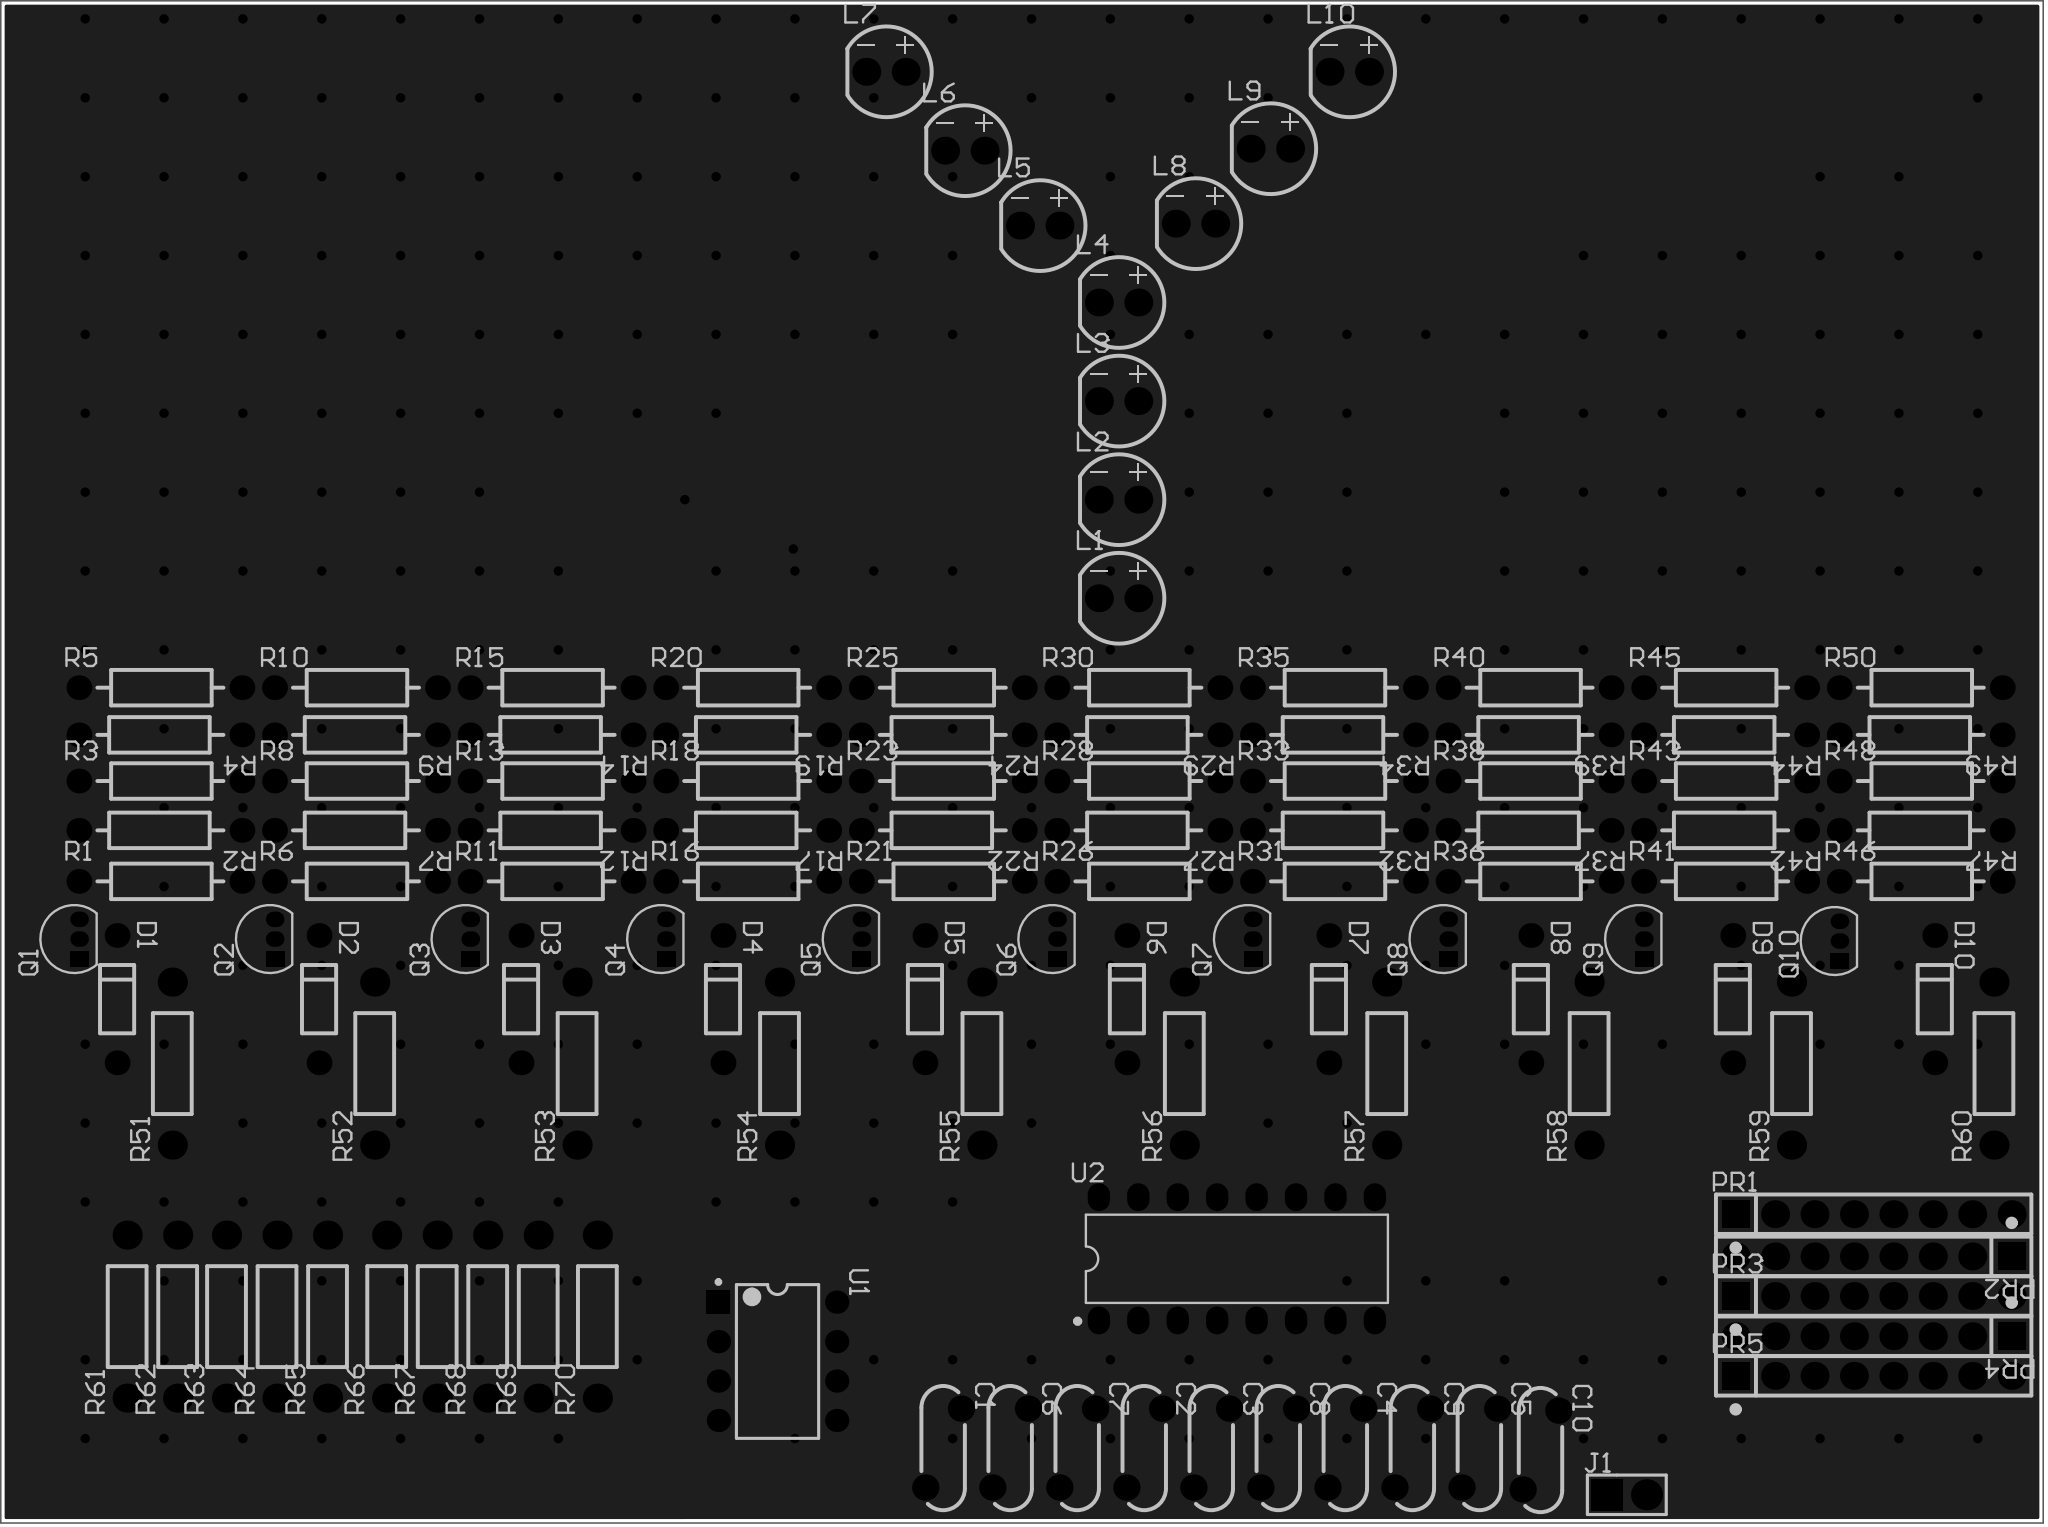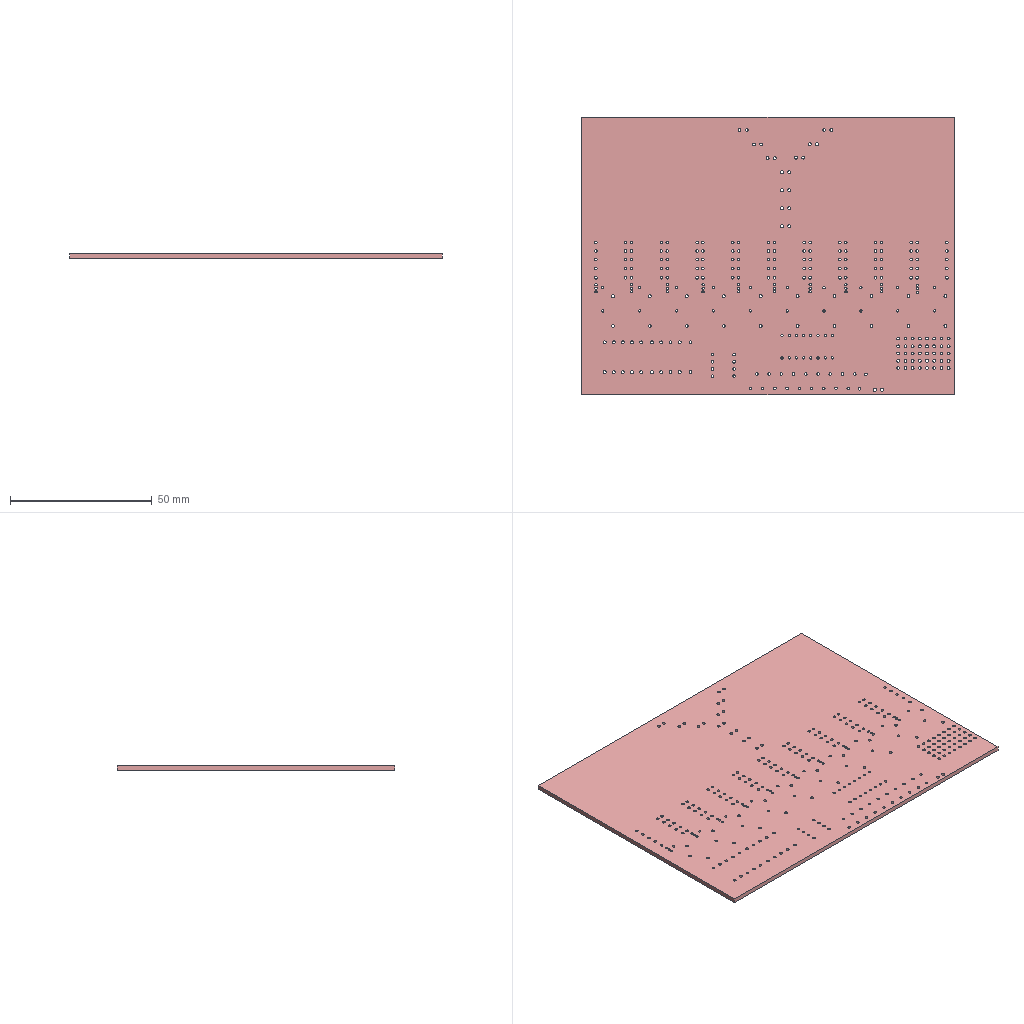Circuit board layout | Altium Designer | box 131.6 x 98 x 1.6 mm
Layer stack:
# Altium Designer layer stack of  (unit mm; dielectric type: 0 none, 1 core, 2 prepreg, 3 surface material)
index,name,kind,layer,copper_thickness_mm,dielectric_type,dielectric_thickness_mm,dielectric_material,dielectric_constant
0,Top Paste Mask Layer,other,,,,,,
1,Top Silkscreen Layer,other,,,,,,
2,Top Solder Mask Layer,dielectric,,,3,0.01,,3.3
3,Top Layer,copper,Top Layer,0.035,,,,
4,Dielectric1,dielectric,,,3,1.51,FR4,4.5
5,Bottom Layer,copper,Bottom Layer,0.035,,,,
6,Bottom Solder Mask Layer,dielectric,,,3,0.01,,3.3
7,Bottom Silkscreen Layer,other,,,,,,
8,Bottom Paste Mask Layer,other,,,,,,
# drill layer pairs: low layer,high layer
drill_pair,Top Layer,Bottom Layer
Part placement:
Designator,Comment,Layer,Footprint,Center-X(mm),Center-Y(mm),Rotation
C1,10nF,TopLayer,CAP-TH_L8.0-W2.8-P5.08-D0.6,143.51,88.9,270
C2,10nF,TopLayer,CAP-TH_L8.0-W2.8-P5.08-D0.6,156.464,88.9,270
C3,10nF,TopLayer,CAP-TH_L8.0-W2.8-P5.08-D0.6,160.782,88.9,270
C4,10nF,TopLayer,CAP-TH_L8.0-W2.8-P5.08-D0.6,169.418,88.9,270
C5,10nF,TopLayer,CAP-TH_L8.0-W2.8-P5.08-D0.6,178.054,88.9,270
C6,10nF,TopLayer,CAP-TH_L8.0-W2.8-P5.08-D0.6,147.828,88.9,270
C7,10nF,TopLayer,CAP-TH_L8.0-W2.8-P5.08-D0.6,152.146,88.9,270
C8,10nF,TopLayer,CAP-TH_L8.0-W2.8-P5.08-D0.6,165.1,88.9,270
C9,10nF,TopLayer,CAP-TH_L8.0-W2.8-P5.08-D0.6,173.736,88.9,270
C10,10nF,TopLayer,CAP-TH_L8.0-W2.8-P5.08-D0.6,181.991,88.773,270
D1,1N4148TR,TopLayer,DO-35_BD2.0-L4.2-P8.20-D0.5-RD,90.297,117.815,270
D2,1N4148TR,TopLayer,DO-35_BD2.0-L4.2-P8.20-D0.5-RD,103.307,117.815,270
D3,1N4148TR,TopLayer,DO-35_BD2.0-L4.2-P8.20-D0.5-RD,116.318,117.815,270
D4,1N4148TR,TopLayer,DO-35_BD2.0-L4.2-P8.20-D0.5-RD,129.328,117.815,270
D5,1N4148TR,TopLayer,DO-35_BD2.0-L4.2-P8.20-D0.5-RD,142.339,117.815,270
D6,1N4148TR,TopLayer,DO-35_BD2.0-L4.2-P8.20-D0.5-RD,155.349,117.815,270
D7,1N4148TR,TopLayer,DO-35_BD2.0-L4.2-P8.20-D0.5-RD,168.36,117.815,270
D8,1N4148TR,TopLayer,DO-35_BD2.0-L4.2-P8.20-D0.5-RD,181.37,117.815,270
D9,1N4148TR,TopLayer,DO-35_BD2.0-L4.2-P8.20-D0.5-RD,194.381,117.815,270
D10,1N4148TR,TopLayer,DO-35_BD2.0-L4.2-P8.20-D0.5-RD,207.391,117.815,270
J1,PZ254V-11-02P,TopLayer,HDR-TH_2P-P2.54-V-M,187.552,85.892,0
L1,XL-502SURD,TopLayer,LED-TH_BD5.9-P2.54-RD_RED,154.813,143.637,0
L2,XL-502SURD,TopLayer,LED-TH_BD5.9-P2.54-RD_RED,154.813,149.987,0
L3,XL-502SURD,TopLayer,LED-TH_BD5.9-P2.54-RD_RED,154.813,156.337,0
L4,XL-502SURD,TopLayer,LED-TH_BD5.9-P2.54-RD_RED,154.813,162.687,0
L5,XL-502SURD,TopLayer,LED-TH_BD5.9-P2.54-RD_RED,149.733,167.64,0
L6,XL-502SURD,TopLayer,LED-TH_BD5.9-P2.54-RD_RED,144.907,172.466,0
L7,XL-502SURD,TopLayer,LED-TH_BD5.9-P2.54-RD_RED,139.827,177.546,0
L8,XL-502SURD,TopLayer,LED-TH_BD5.9-P2.54-RD_RED,159.766,167.767,0
L9,XL-502SURD,TopLayer,LED-TH_BD5.9-P2.54-RD_RED,164.592,172.593,0
L10,XL-502SURD,TopLayer,LED-TH_BD5.9-P2.54-RD_RED,169.672,177.546,0
PR1,10kΩ,TopLayer,RES-ARRAY-TH_8P-L20.3-W2.5-P2.54,203.454,103.964,0
PR2,10kΩ,TopLayer,RES-ARRAY-TH_8P-L20.3-W2.5-P2.54,203.454,101.247,180
PR3,10kΩ,TopLayer,RES-ARRAY-TH_8P-L20.3-W2.5-P2.54,203.454,98.695,0
PR4,10kΩ,TopLayer,RES-ARRAY-TH_8P-L20.3-W2.5-P2.54,203.454,96.105,180
PR5,10kΩ,TopLayer,RES-ARRAY-TH_8P-L20.3-W2.5-P2.54,203.454,93.552,0
Q1,S8050,TopLayer,TO-92-3_L4.5-W3.5-P1.27-L,87.88,121.686,90
Q2,S8050,TopLayer,TO-92-3_L4.5-W3.5-P1.27-L,100.48,121.686,90
Q3,S8050,TopLayer,TO-92-3_L4.5-W3.5-P1.27-L,113.08,121.686,90
Q4,S8050,TopLayer,TO-92-3_L4.5-W3.5-P1.27-L,125.68,121.686,90
Q5,S8050,TopLayer,TO-92-3_L4.5-W3.5-P1.27-L,138.28,121.686,90
Q6,S8050,TopLayer,TO-92-3_L4.5-W3.5-P1.27-L,150.881,121.686,90
Q7,S8050,TopLayer,TO-92-3_L4.5-W3.5-P1.27-L,163.481,121.686,90
Q8,S8050,TopLayer,TO-92-3_L4.5-W3.5-P1.27-L,176.081,121.686,90
Q9,S8050,TopLayer,TO-92-3_L4.5-W3.5-P1.27-L,188.681,121.686,90
Q10,S8050,TopLayer,TO-92-3_L4.5-W3.5-P1.27-L,201.281,121.559,90
R1,100Ω,TopLayer,RES-TH_BD2.2-L6.5-P10.50-D0.6,93.087,125.402,0
R2,100Ω,TopLayer,RES-TH_BD2.2-L6.5-P10.50-D0.6,93.087,128.687,180
R3,100Ω,TopLayer,RES-TH_BD2.2-L6.5-P10.50-D0.6,93.087,131.865,0
R4,100Ω,TopLayer,RES-TH_BD2.2-L6.5-P10.50-D0.6,93.087,134.837,180
R5,100Ω,TopLayer,RES-TH_BD2.2-L6.5-P10.50-D0.6,93.087,137.877,0
R6,100Ω,TopLayer,RES-TH_BD2.2-L6.5-P10.50-D0.6,105.687,125.402,0
R7,100Ω,TopLayer,RES-TH_BD2.2-L6.5-P10.50-D0.6,105.687,128.687,180
R8,100Ω,TopLayer,RES-TH_BD2.2-L6.5-P10.50-D0.6,105.687,131.865,0
R9,100Ω,TopLayer,RES-TH_BD2.2-L6.5-P10.50-D0.6,105.687,134.837,180
R10,100Ω,TopLayer,RES-TH_BD2.2-L6.5-P10.50-D0.6,105.687,137.877,0
R11,100Ω,TopLayer,RES-TH_BD2.2-L6.5-P10.50-D0.6,118.287,125.402,0
R12,100Ω,TopLayer,RES-TH_BD2.2-L6.5-P10.50-D0.6,118.287,128.687,180
R13,100Ω,TopLayer,RES-TH_BD2.2-L6.5-P10.50-D0.6,118.287,131.865,0
R14,100Ω,TopLayer,RES-TH_BD2.2-L6.5-P10.50-D0.6,118.287,134.837,180
R15,100Ω,TopLayer,RES-TH_BD2.2-L6.5-P10.50-D0.6,118.287,137.877,0
R16,100Ω,TopLayer,RES-TH_BD2.2-L6.5-P10.50-D0.6,130.887,125.402,0
R17,100Ω,TopLayer,RES-TH_BD2.2-L6.5-P10.50-D0.6,130.887,128.687,180
R18,100Ω,TopLayer,RES-TH_BD2.2-L6.5-P10.50-D0.6,130.887,131.865,0
R19,100Ω,TopLayer,RES-TH_BD2.2-L6.5-P10.50-D0.6,130.887,134.837,180
R20,100Ω,TopLayer,RES-TH_BD2.2-L6.5-P10.50-D0.6,130.887,137.877,0
R21,100Ω,TopLayer,RES-TH_BD2.2-L6.5-P10.50-D0.6,143.487,125.402,0
R22,100Ω,TopLayer,RES-TH_BD2.2-L6.5-P10.50-D0.6,143.488,128.687,180
R23,100Ω,TopLayer,RES-TH_BD2.2-L6.5-P10.50-D0.6,143.487,131.865,0
R24,100Ω,TopLayer,RES-TH_BD2.2-L6.5-P10.50-D0.6,143.488,134.837,180
R25,100Ω,TopLayer,RES-TH_BD2.2-L6.5-P10.50-D0.6,143.487,137.877,0
R26,100Ω,TopLayer,RES-TH_BD2.2-L6.5-P10.50-D0.6,156.088,125.402,0
R27,100Ω,TopLayer,RES-TH_BD2.2-L6.5-P10.50-D0.6,156.088,128.687,180
R28,100Ω,TopLayer,RES-TH_BD2.2-L6.5-P10.50-D0.6,156.088,131.865,0
R29,100Ω,TopLayer,RES-TH_BD2.2-L6.5-P10.50-D0.6,156.088,134.837,180
R30,100Ω,TopLayer,RES-TH_BD2.2-L6.5-P10.50-D0.6,156.088,137.877,0
R31,100Ω,TopLayer,RES-TH_BD2.2-L6.5-P10.50-D0.6,168.688,125.402,0
R32,100Ω,TopLayer,RES-TH_BD2.2-L6.5-P10.50-D0.6,168.688,128.687,180
R33,100Ω,TopLayer,RES-TH_BD2.2-L6.5-P10.50-D0.6,168.688,131.865,0
R34,100Ω,TopLayer,RES-TH_BD2.2-L6.5-P10.50-D0.6,168.688,134.837,180
R35,100Ω,TopLayer,RES-TH_BD2.2-L6.5-P10.50-D0.6,168.688,137.877,0
R36,100Ω,TopLayer,RES-TH_BD2.2-L6.5-P10.50-D0.6,181.288,125.402,0
R37,100Ω,TopLayer,RES-TH_BD2.2-L6.5-P10.50-D0.6,181.288,128.687,180
R38,100Ω,TopLayer,RES-TH_BD2.2-L6.5-P10.50-D0.6,181.288,131.865,0
R39,100Ω,TopLayer,RES-TH_BD2.2-L6.5-P10.50-D0.6,181.288,134.837,180
R40,100Ω,TopLayer,RES-TH_BD2.2-L6.5-P10.50-D0.6,181.288,137.877,0
R41,100Ω,TopLayer,RES-TH_BD2.2-L6.5-P10.50-D0.6,193.888,125.402,0
R42,100Ω,TopLayer,RES-TH_BD2.2-L6.5-P10.50-D0.6,193.888,128.687,180
R43,100Ω,TopLayer,RES-TH_BD2.2-L6.5-P10.50-D0.6,193.888,131.865,0
R44,100Ω,TopLayer,RES-TH_BD2.2-L6.5-P10.50-D0.6,193.888,134.837,180
R45,100Ω,TopLayer,RES-TH_BD2.2-L6.5-P10.50-D0.6,193.888,137.877,0
R46,100Ω,TopLayer,RES-TH_BD2.2-L6.5-P10.50-D0.6,206.488,125.402,0
R47,100Ω,TopLayer,RES-TH_BD2.2-L6.5-P10.50-D0.6,206.488,128.687,180
R48,100Ω,TopLayer,RES-TH_BD2.2-L6.5-P10.50-D0.6,206.488,131.865,0
R49,100Ω,TopLayer,RES-TH_BD2.2-L6.5-P10.50-D0.6,206.488,134.837,180
R50,100Ω,TopLayer,RES-TH_BD2.2-L6.5-P10.50-D0.6,206.488,137.877,0
R51,1kΩ,TopLayer,RES-TH_BD2.5-L6.5-P10.50-D0.6,93.853,113.665,90
R52,1kΩ,TopLayer,RES-TH_BD2.5-L6.5-P10.50-D0.6,106.892,113.665,90
R53,1kΩ,TopLayer,RES-TH_BD2.5-L6.5-P10.50-D0.6,119.93,113.665,90
R54,1kΩ,TopLayer,RES-TH_BD2.5-L6.5-P10.50-D0.6,132.969,113.665,90
R55,1kΩ,TopLayer,RES-TH_BD2.5-L6.5-P10.50-D0.6,146.008,113.665,90
R56,1kΩ,TopLayer,RES-TH_BD2.5-L6.5-P10.50-D0.6,159.046,113.665,90
R57,1kΩ,TopLayer,RES-TH_BD2.5-L6.5-P10.50-D0.6,172.085,113.665,90
R58,1kΩ,TopLayer,RES-TH_BD2.5-L6.5-P10.50-D0.6,185.124,113.665,90
R59,1kΩ,TopLayer,RES-TH_BD2.5-L6.5-P10.50-D0.6,198.162,113.665,90
R60,1kΩ,TopLayer,RES-TH_BD2.5-L6.5-P10.50-D0.6,211.201,113.665,90
R61,1kΩ,TopLayer,RES-TH_BD2.5-L6.5-P10.50-D0.6,90.944,97.368,90
R62,1kΩ,TopLayer,RES-TH_BD2.5-L6.5-P10.50-D0.6,94.198,97.368,90
R63,1kΩ,TopLayer,RES-TH_BD2.5-L6.5-P10.50-D0.6,97.346,97.368,90
R64,1kΩ,TopLayer,RES-TH_BD2.5-L6.5-P10.50-D0.6,100.6,97.368,90
R65,1kΩ,TopLayer,RES-TH_BD2.5-L6.5-P10.50-D0.6,103.853,97.368,90
R66,1kΩ,TopLayer,RES-TH_BD2.5-L6.5-P10.50-D0.6,107.663,97.368,90
R67,1kΩ,TopLayer,RES-TH_BD2.5-L6.5-P10.50-D0.6,110.918,97.368,90
R68,1kΩ,TopLayer,RES-TH_BD2.5-L6.5-P10.50-D0.6,114.172,97.368,90
R69,1kΩ,TopLayer,RES-TH_BD2.5-L6.5-P10.50-D0.6,117.426,97.368,90
R70,1kΩ,TopLayer,RES-TH_BD2.5-L6.5-P10.50-D0.6,121.236,97.368,90
U1,NE555P,TopLayer,DIP-8_L9.8-W6.6-P2.54-LS7.6-BL,132.842,94.488,270
U2,CD4017CN,TopLayer,PDIP-16_L19.3-W6.4-P2.54-LS7.94-BL,162.433,101.092,0
Pad and via stacks:
# Altium Designer via and pad stacks of  (unit mm). Each distinct definition once, with the count of objects using it.
# via: kind,start_layer,end_layer,hole_mm,diameter_mm,mode(0 simple;1 top-mid-bottom;2 full stack),diameter_per_layer,count,example_net
# pad: kind,layer,hole_mm,hole_type(0 round;1 square;2 slot),plating,top_size,top_shape(1 round;2 rect;3 octagon;9 rounded rect),mid_size,bottom_size,mode,footprint,size_per_layer,count,example
pad,Multi-Layer,0.9,0,plated,1.7x1.7,1,1.7x1.7,1.7x1.7,0,CAP-TH_L8.0-W2.8-P5.08-D0.6,,20,C1.1
pad,Multi-Layer,0.8,0,plated,1.6x1.6,1,1.6x1.6,1.6x1.6,0,DO-35_BD2.0-L4.2-P8.20-D0.5-RD,,20,D1.2
pad,Multi-Layer,1.2,0,plated,2x2,2,2x2,2x2,0,HDR-TH_2P-P2.54-V-M,,1,J1.1
pad,Multi-Layer,1.2,0,plated,2x2,1,2x2,2x2,0,HDR-TH_2P-P2.54-V-M,,1,J1.2
pad,Multi-Layer,1,0,plated,1.8x1.8,1,1.8x1.8,1.8x1.8,0,LED-TH_BD5.9-P2.54-RD_RED,,20,L1.2
pad,Multi-Layer,1,0,plated,1.8x1.8,2,1.8x1.8,1.8x1.8,0,RES-ARRAY-TH_8P-L20.3-W2.5-P2.54,,5,PR1.1
pad,Multi-Layer,1,0,plated,1.8x1.8,1,1.8x1.8,1.8x1.8,0,RES-ARRAY-TH_8P-L20.3-W2.5-P2.54,,35,PR1.2
pad,Multi-Layer,0.7,2,plated,1x1.2,2,1x1.2,1x1.2,0,TO-92-3_L4.5-W3.5-P1.27-L,,10,Q1.1
pad,Multi-Layer,0.7,2,plated,1x1.2,1,1x1.2,1x1.2,0,TO-92-3_L4.5-W3.5-P1.27-L,,20,Q1.2
pad,Multi-Layer,0.9144,0,plated,1.6x1.6,1,1.6x1.6,1.6x1.6,0,RES-TH_BD2.2-L6.5-P10.50-D0.6,,100,R1.1
pad,Multi-Layer,1,0,plated,1.88x1.88,1,1.88x1.88,1.88x1.88,0,RES-TH_BD2.5-L6.5-P10.50-D0.6,,40,R51.1
pad,Multi-Layer,0.9,0,plated,1.5x1.5,2,1.5x1.5,1.5x1.5,0,DIP-8_L9.8-W6.6-P2.54-LS7.6-BL,,1,U1.1
pad,Multi-Layer,0.9,0,plated,1.5x1.5,1,1.5x1.5,1.5x1.5,0,DIP-8_L9.8-W6.6-P2.54-LS7.6-BL,,7,U1.2
pad,Multi-Layer,0.8,0,plated,1.44x1.8,1,1.44x1.8,1.44x1.8,0,PDIP-16_L19.3-W6.4-P2.54-LS7.94-BL,,16,U2.1
via,Top Layer,Bottom Layer,0.3048,0.61,0,,345,$1N7169
Copper pours:
name,layer,net,type(0 solid;1 hatched;2 none)
Bottom Layer-GND,Bottom Layer,GND,0
Top Layer-GND,Top Layer,GND,0